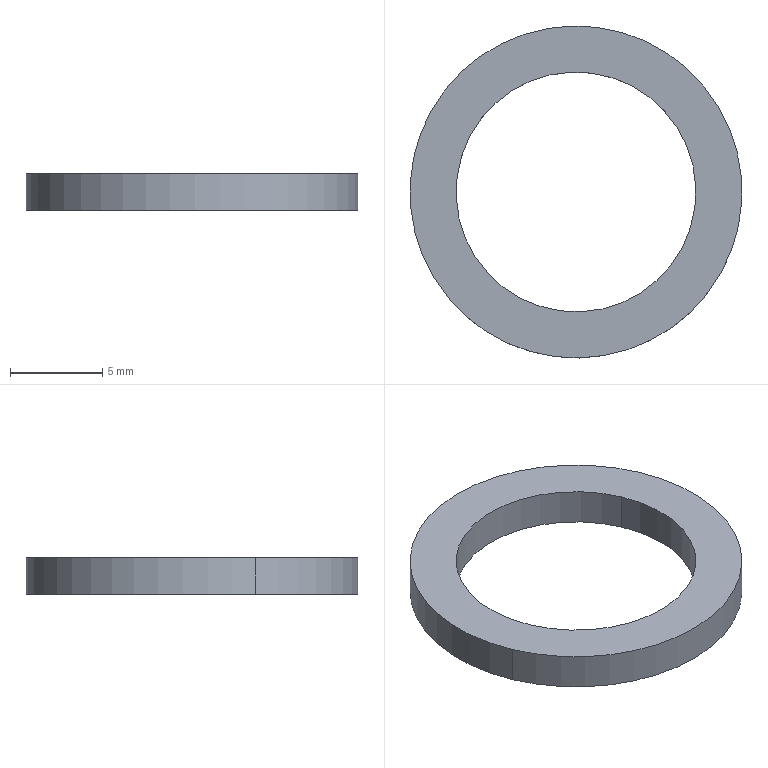Part | SolidWorks | features BaseBody 1 | 1 solid | 6 faces | box 18 x 18 x 2 mm | volume 243.473 mm3 | cylinder 4 | plane 2 | commonest cylinder face diameters 13 x2 18 x2
STEP:
#1=CARTESIAN_POINT('',(-52.776,-8.551,-256.55));
#2=VERTEX_POINT('',#1);
#3=CARTESIAN_POINT('',(-36.149,-1.656,-256.55));
#4=VERTEX_POINT('',#3);
#5=CARTESIAN_POINT('',(-44.463,-5.104,-256.55));
#6=DIRECTION('',(0.,0.,-1.));
#7=DIRECTION('',(-0.9237,-0.383,0.));
#8=AXIS2_PLACEMENT_3D('',#5,#6,#7);
#9=CIRCLE('',#8,9.);
#10=EDGE_CURVE('',#2,#4,#9,.T.);
#11=ORIENTED_EDGE('',*,*,#10,.F.);
#12=CARTESIAN_POINT('',(-52.776,-8.551,-254.55));
#13=VERTEX_POINT('',#12);
#14=CARTESIAN_POINT('',(-52.776,-8.551,-256.55));
#15=DIRECTION('',(0.,0.,1.));
#16=VECTOR('',#15,1000.);
#17=LINE('',#14,#16);
#18=EDGE_CURVE('',#2,#13,#17,.T.);
#19=ORIENTED_EDGE('',*,*,#18,.T.);
#20=CARTESIAN_POINT('',(-36.149,-1.656,-254.55));
#21=VERTEX_POINT('',#20);
#22=CARTESIAN_POINT('',(-44.463,-5.104,-254.55));
#23=DIRECTION('',(0.,0.,-1.));
#24=DIRECTION('',(-0.9237,-0.383,0.));
#25=AXIS2_PLACEMENT_3D('',#22,#23,#24);
#26=CIRCLE('',#25,9.);
#27=EDGE_CURVE('',#13,#21,#26,.T.);
#28=ORIENTED_EDGE('',*,*,#27,.T.);
#29=CARTESIAN_POINT('',(-36.149,-1.656,-256.55));
#30=DIRECTION('',(0.,0.,1.));
#31=VECTOR('',#30,1000.);
#32=LINE('',#29,#31);
#33=EDGE_CURVE('',#4,#21,#32,.T.);
#34=ORIENTED_EDGE('',*,*,#33,.F.);
#35=EDGE_LOOP('',(#11,#19,#28,#34));
#36=FACE_OUTER_BOUND('',#35,.T.);
#37=CARTESIAN_POINT('',(-44.463,-5.104,-256.55));
#38=DIRECTION('',(0.,0.,1.));
#39=DIRECTION('',(0.9237,0.383,0.));
#40=AXIS2_PLACEMENT_3D('',#37,#38,#39);
#41=CYLINDRICAL_SURFACE('',#40,9.);
#42=ADVANCED_FACE('',(#36),#41,.T.);
#43=CARTESIAN_POINT('',(-38.459,-2.614,-256.55));
#44=VERTEX_POINT('',#43);
#45=CARTESIAN_POINT('',(-50.467,-7.594,-256.55));
#46=VERTEX_POINT('',#45);
#47=CARTESIAN_POINT('',(-44.463,-5.104,-256.55));
#48=DIRECTION('',(0.,0.,-1.));
#49=DIRECTION('',(-0.9237,-0.383,0.));
#50=AXIS2_PLACEMENT_3D('',#47,#48,#49);
#51=CIRCLE('',#50,6.5);
#52=EDGE_CURVE('',#44,#46,#51,.T.);
#53=ORIENTED_EDGE('',*,*,#52,.T.);
#54=CARTESIAN_POINT('',(-50.467,-7.594,-254.55));
#55=VERTEX_POINT('',#54);
#56=CARTESIAN_POINT('',(-50.467,-7.594,-256.55));
#57=DIRECTION('',(0.,0.,1.));
#58=VECTOR('',#57,1000.);
#59=LINE('',#56,#58);
#60=EDGE_CURVE('',#46,#55,#59,.T.);
#61=ORIENTED_EDGE('',*,*,#60,.T.);
#62=CARTESIAN_POINT('',(-38.459,-2.614,-254.55));
#63=VERTEX_POINT('',#62);
#64=CARTESIAN_POINT('',(-44.463,-5.104,-254.55));
#65=DIRECTION('',(0.,0.,-1.));
#66=DIRECTION('',(-0.9237,-0.383,0.));
#67=AXIS2_PLACEMENT_3D('',#64,#65,#66);
#68=CIRCLE('',#67,6.5);
#69=EDGE_CURVE('',#63,#55,#68,.T.);
#70=ORIENTED_EDGE('',*,*,#69,.F.);
#71=CARTESIAN_POINT('',(-38.459,-2.614,-256.55));
#72=DIRECTION('',(0.,0.,1.));
#73=VECTOR('',#72,1000.);
#74=LINE('',#71,#73);
#75=EDGE_CURVE('',#44,#63,#74,.T.);
#76=ORIENTED_EDGE('',*,*,#75,.F.);
#77=EDGE_LOOP('',(#53,#61,#70,#76));
#78=FACE_OUTER_BOUND('',#77,.T.);
#79=CARTESIAN_POINT('',(-44.463,-5.104,-256.55));
#80=DIRECTION('',(0.,0.,1.));
#81=DIRECTION('',(0.9237,0.383,0.));
#82=AXIS2_PLACEMENT_3D('',#79,#80,#81);
#83=CYLINDRICAL_SURFACE('',#82,6.5);
#84=ADVANCED_FACE('',(#78),#83,.F.);
#85=ORIENTED_EDGE('',*,*,#60,.F.);
#86=CARTESIAN_POINT('',(-44.463,-5.104,-256.55));
#87=DIRECTION('',(0.,0.,-1.));
#88=DIRECTION('',(-0.9237,-0.383,0.));
#89=AXIS2_PLACEMENT_3D('',#86,#87,#88);
#90=CIRCLE('',#89,6.5);
#91=EDGE_CURVE('',#46,#44,#90,.T.);
#92=ORIENTED_EDGE('',*,*,#91,.T.);
#93=ORIENTED_EDGE('',*,*,#75,.T.);
#94=CARTESIAN_POINT('',(-44.463,-5.104,-254.55));
#95=DIRECTION('',(0.,0.,-1.));
#96=DIRECTION('',(-0.9237,-0.383,0.));
#97=AXIS2_PLACEMENT_3D('',#94,#95,#96);
#98=CIRCLE('',#97,6.5);
#99=EDGE_CURVE('',#55,#63,#98,.T.);
#100=ORIENTED_EDGE('',*,*,#99,.F.);
#101=EDGE_LOOP('',(#85,#92,#93,#100));
#102=FACE_OUTER_BOUND('',#101,.T.);
#103=CARTESIAN_POINT('',(-44.463,-5.104,-256.55));
#104=DIRECTION('',(0.,0.,1.));
#105=DIRECTION('',(0.9237,0.383,0.));
#106=AXIS2_PLACEMENT_3D('',#103,#104,#105);
#107=CYLINDRICAL_SURFACE('',#106,6.5);
#108=ADVANCED_FACE('',(#102),#107,.F.);
#109=ORIENTED_EDGE('',*,*,#18,.F.);
#110=CARTESIAN_POINT('',(-44.463,-5.104,-256.55));
#111=DIRECTION('',(0.,0.,-1.));
#112=DIRECTION('',(-0.9237,-0.383,0.));
#113=AXIS2_PLACEMENT_3D('',#110,#111,#112);
#114=CIRCLE('',#113,9.);
#115=EDGE_CURVE('',#4,#2,#114,.T.);
#116=ORIENTED_EDGE('',*,*,#115,.F.);
#117=ORIENTED_EDGE('',*,*,#33,.T.);
#118=CARTESIAN_POINT('',(-44.463,-5.104,-254.55));
#119=DIRECTION('',(0.,0.,-1.));
#120=DIRECTION('',(-0.9237,-0.383,0.));
#121=AXIS2_PLACEMENT_3D('',#118,#119,#120);
#122=CIRCLE('',#121,9.);
#123=EDGE_CURVE('',#21,#13,#122,.T.);
#124=ORIENTED_EDGE('',*,*,#123,.T.);
#125=EDGE_LOOP('',(#109,#116,#117,#124));
#126=FACE_OUTER_BOUND('',#125,.T.);
#127=CARTESIAN_POINT('',(-44.463,-5.104,-256.55));
#128=DIRECTION('',(0.,0.,1.));
#129=DIRECTION('',(0.9237,0.383,0.));
#130=AXIS2_PLACEMENT_3D('',#127,#128,#129);
#131=CYLINDRICAL_SURFACE('',#130,9.);
#132=ADVANCED_FACE('',(#126),#131,.T.);
#133=ORIENTED_EDGE('',*,*,#69,.T.);
#134=ORIENTED_EDGE('',*,*,#99,.T.);
#135=EDGE_LOOP('',(#133,#134));
#136=FACE_BOUND('',#135,.T.);
#137=ORIENTED_EDGE('',*,*,#123,.F.);
#138=ORIENTED_EDGE('',*,*,#27,.F.);
#139=EDGE_LOOP('',(#137,#138));
#140=FACE_OUTER_BOUND('',#139,.T.);
#141=CARTESIAN_POINT('',(-44.463,-5.104,-254.55));
#142=DIRECTION('',(0.,0.,-1.));
#143=DIRECTION('',(0.,-1.,0.));
#144=AXIS2_PLACEMENT_3D('',#141,#142,#143);
#145=PLANE('',#144);
#146=ADVANCED_FACE('',(#136,#140),#145,.F.);
#147=ORIENTED_EDGE('',*,*,#52,.F.);
#148=ORIENTED_EDGE('',*,*,#91,.F.);
#149=EDGE_LOOP('',(#147,#148));
#150=FACE_BOUND('',#149,.T.);
#151=ORIENTED_EDGE('',*,*,#115,.T.);
#152=ORIENTED_EDGE('',*,*,#10,.T.);
#153=EDGE_LOOP('',(#151,#152));
#154=FACE_OUTER_BOUND('',#153,.T.);
#155=CARTESIAN_POINT('',(-44.463,-5.104,-256.55));
#156=DIRECTION('',(0.,0.,-1.));
#157=DIRECTION('',(0.,-1.,0.));
#158=AXIS2_PLACEMENT_3D('',#155,#156,#157);
#159=PLANE('',#158);
#160=ADVANCED_FACE('',(#150,#154),#159,.T.);
#161=CLOSED_SHELL('',(#42,#84,#108,#132,#146,#160));
#162=MANIFOLD_SOLID_BREP('',#161);
#163=CARTESIAN_POINT('',(0.,0.,0.));
#164=DIRECTION('',(0.,0.,1.));
#165=DIRECTION('',(1.,0.,0.));
#166=AXIS2_PLACEMENT_3D('',#163,#164,#165);
#167=(LENGTH_UNIT()NAMED_UNIT(*)SI_UNIT(.MILLI.,.METRE.));
#168=UNCERTAINTY_MEASURE_WITH_UNIT(LENGTH_MEASURE(0.00001),#167,'','');
#169=(NAMED_UNIT(*)PLANE_ANGLE_UNIT()SI_UNIT($,.RADIAN.));
#170=(NAMED_UNIT(*)SI_UNIT($,.STERADIAN.)SOLID_ANGLE_UNIT());
#171=(GEOMETRIC_REPRESENTATION_CONTEXT(3)GLOBAL_UNCERTAINTY_ASSIGNED_CONTEXT((#168))GLOBAL_UNIT_ASSIGNED_CONTEXT((#167,#169,#170))REPRESENTATION_CONTEXT('',''));
#172=ADVANCED_BREP_SHAPE_REPRESENTATION('',(#162,#166),#171);